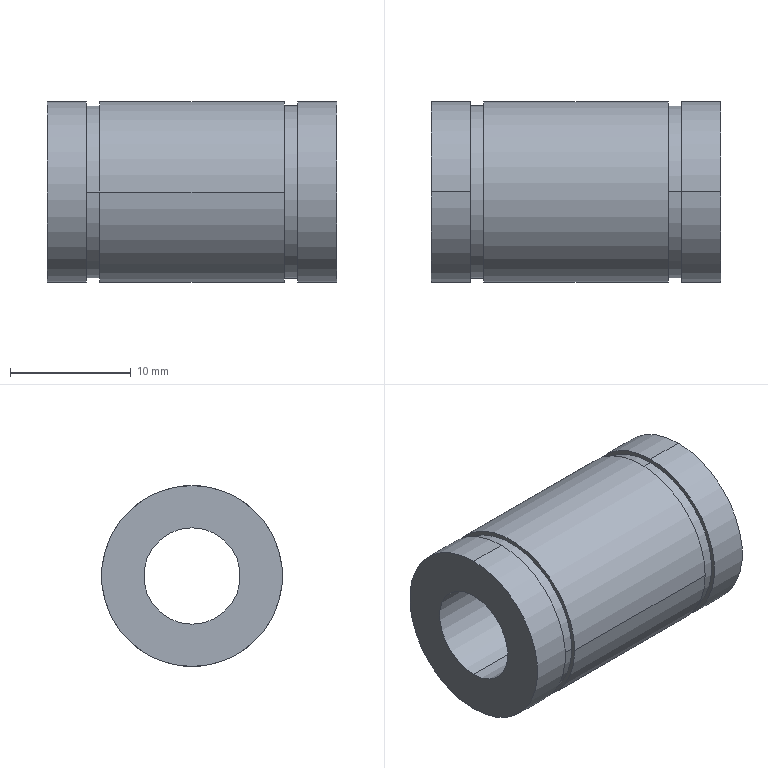Part | STEP file | Linear bearing LMU8 | 1 solid | 18 faces | box 24 x 15 x 15 mm | volume 2999 mm3 | cylinder 12 | plane 6 | commonest cylinder face diameters 15 x6 14.3 x4 8 x2
STEP:
#1=CARTESIAN_POINT('',(0.,0.,0.));
#2=DIRECTION('',(0.,0.,1.));
#3=DIRECTION('',(1.,0.,0.));
#4=AXIS2_PLACEMENT_3D('',#1,#2,#3);
#5=CARTESIAN_POINT('',(8.75,0.,-7.15));
#6=VERTEX_POINT('',#5);
#7=CARTESIAN_POINT('',(8.75,0.,7.15));
#8=VERTEX_POINT('',#7);
#9=CARTESIAN_POINT('',(8.75,0.,0.));
#10=DIRECTION('',(1.,0.,0.));
#11=DIRECTION('',(0.,0.,1.));
#12=AXIS2_PLACEMENT_3D('',#9,#10,#11);
#13=CIRCLE('',#12,7.15);
#14=CARTESIAN_POINT('',(8.75,0.,0.));
#15=DIRECTION('',(-1.,0.,0.));
#16=DIRECTION('',(0.,0.,1.));
#17=AXIS2_PLACEMENT_3D('',#14,#15,#16);
#18=CYLINDRICAL_SURFACE('',#17,7.15);
#19=CARTESIAN_POINT('',(6.283,0.));
#20=DIRECTION('',(-1.,0.));
#21=VECTOR('',#20,1.);
#22=LINE('',#19,#21);
#23=(GEOMETRIC_REPRESENTATION_CONTEXT(2)PARAMETRIC_REPRESENTATION_CONTEXT()REPRESENTATION_CONTEXT('',''));
#24=DEFINITIONAL_REPRESENTATION('',(#22),#23);
#25=PCURVE('',#18,#24);
#26=CARTESIAN_POINT('',(8.75,-7.59,-7.59));
#27=DIRECTION('',(-1.,0.,0.));
#28=DIRECTION('',(0.,0.,1.));
#29=AXIS2_PLACEMENT_3D('',#26,#27,#28);
#30=PLANE('',#29);
#31=CARTESIAN_POINT('',(14.74,7.59));
#32=CARTESIAN_POINT('',(14.74,-4.794));
#33=CARTESIAN_POINT('',(4.015,1.398));
#34=CARTESIAN_POINT('',(-6.71,7.59));
#35=CARTESIAN_POINT('',(4.015,13.782));
#36=CARTESIAN_POINT('',(14.74,19.974));
#37=CARTESIAN_POINT('',(14.74,7.59));
#38=(BOUNDED_CURVE()B_SPLINE_CURVE(2,(#31,#32,#33,#34,#35,#36,#37),.UNSPECIFIED.,.T.,.F.)B_SPLINE_CURVE_WITH_KNOTS((1,2,2,2,2,1),(-2.094,0.,2.094,4.189,6.283,8.378),.UNSPECIFIED.)CURVE()GEOMETRIC_REPRESENTATION_ITEM()RATIONAL_B_SPLINE_CURVE((1.,0.5,1.,0.5,1.,0.5,1.))REPRESENTATION_ITEM(''));
#39=(GEOMETRIC_REPRESENTATION_CONTEXT(2)PARAMETRIC_REPRESENTATION_CONTEXT()REPRESENTATION_CONTEXT('',''));
#40=DEFINITIONAL_REPRESENTATION('',(#38),#39);
#41=PCURVE('',#30,#40);
#42=SURFACE_CURVE('',#13,(#25,#41),.PCURVE_S1.);
#43=EDGE_CURVE('',#6,#8,#42,.T.);
#44=ORIENTED_EDGE('',*,*,#43,.F.);
#45=CARTESIAN_POINT('',(7.65,0.,-7.15));
#46=VERTEX_POINT('',#45);
#47=CARTESIAN_POINT('',(8.75,0.,-7.15));
#48=DIRECTION('',(-1.,0.,0.));
#49=VECTOR('',#48,1.);
#50=LINE('',#47,#49);
#51=CARTESIAN_POINT('',(3.142,0.));
#52=DIRECTION('',(0.,1.));
#53=VECTOR('',#52,1.);
#54=LINE('',#51,#53);
#55=(GEOMETRIC_REPRESENTATION_CONTEXT(2)PARAMETRIC_REPRESENTATION_CONTEXT()REPRESENTATION_CONTEXT('',''));
#56=DEFINITIONAL_REPRESENTATION('',(#54),#55);
#57=PCURVE('',#18,#56);
#58=CARTESIAN_POINT('',(8.75,0.,0.));
#59=DIRECTION('',(-1.,0.,0.));
#60=DIRECTION('',(0.,0.,1.));
#61=AXIS2_PLACEMENT_3D('',#58,#59,#60);
#62=CYLINDRICAL_SURFACE('',#61,7.15);
#63=CARTESIAN_POINT('',(3.142,0.));
#64=DIRECTION('',(0.,1.));
#65=VECTOR('',#64,1.);
#66=LINE('',#63,#65);
#67=(GEOMETRIC_REPRESENTATION_CONTEXT(2)PARAMETRIC_REPRESENTATION_CONTEXT()REPRESENTATION_CONTEXT('',''));
#68=DEFINITIONAL_REPRESENTATION('',(#66),#67);
#69=PCURVE('',#62,#68);
#70=SURFACE_CURVE('',#50,(#57,#69),.PCURVE_S1.);
#71=EDGE_CURVE('',#6,#46,#70,.T.);
#72=ORIENTED_EDGE('',*,*,#71,.T.);
#73=CARTESIAN_POINT('',(7.65,0.,7.15));
#74=VERTEX_POINT('',#73);
#75=CARTESIAN_POINT('',(7.65,0.,0.));
#76=DIRECTION('',(-1.,0.,0.));
#77=DIRECTION('',(0.,0.,1.));
#78=AXIS2_PLACEMENT_3D('',#75,#76,#77);
#79=CIRCLE('',#78,7.15);
#80=CARTESIAN_POINT('',(0.,1.1));
#81=DIRECTION('',(1.,0.));
#82=VECTOR('',#81,1.);
#83=LINE('',#80,#82);
#84=(GEOMETRIC_REPRESENTATION_CONTEXT(2)PARAMETRIC_REPRESENTATION_CONTEXT()REPRESENTATION_CONTEXT('',''));
#85=DEFINITIONAL_REPRESENTATION('',(#83),#84);
#86=PCURVE('',#18,#85);
#87=CARTESIAN_POINT('',(7.65,-7.59,7.59));
#88=DIRECTION('',(1.,0.,0.));
#89=DIRECTION('',(0.,0.,-1.));
#90=AXIS2_PLACEMENT_3D('',#87,#88,#89);
#91=PLANE('',#90);
#92=CARTESIAN_POINT('',(0.44,7.59));
#93=CARTESIAN_POINT('',(0.44,19.974));
#94=CARTESIAN_POINT('',(11.165,13.782));
#95=CARTESIAN_POINT('',(21.89,7.59));
#96=CARTESIAN_POINT('',(11.165,1.398));
#97=CARTESIAN_POINT('',(0.44,-4.794));
#98=CARTESIAN_POINT('',(0.44,7.59));
#99=(BOUNDED_CURVE()B_SPLINE_CURVE(2,(#92,#93,#94,#95,#96,#97,#98),.UNSPECIFIED.,.T.,.F.)B_SPLINE_CURVE_WITH_KNOTS((1,2,2,2,2,1),(-2.094,0.,2.094,4.189,6.283,8.378),.UNSPECIFIED.)CURVE()GEOMETRIC_REPRESENTATION_ITEM()RATIONAL_B_SPLINE_CURVE((1.,0.5,1.,0.5,1.,0.5,1.))REPRESENTATION_ITEM(''));
#100=(GEOMETRIC_REPRESENTATION_CONTEXT(2)PARAMETRIC_REPRESENTATION_CONTEXT()REPRESENTATION_CONTEXT('',''));
#101=DEFINITIONAL_REPRESENTATION('',(#99),#100);
#102=PCURVE('',#91,#101);
#103=SURFACE_CURVE('',#79,(#86,#102),.PCURVE_S1.);
#104=EDGE_CURVE('',#74,#46,#103,.T.);
#105=ORIENTED_EDGE('',*,*,#104,.F.);
#106=CARTESIAN_POINT('',(8.75,0.,7.15));
#107=DIRECTION('',(-1.,0.,0.));
#108=VECTOR('',#107,1.);
#109=LINE('',#106,#108);
#110=CARTESIAN_POINT('',(0.,0.));
#111=DIRECTION('',(0.,1.));
#112=VECTOR('',#111,1.);
#113=LINE('',#110,#112);
#114=(GEOMETRIC_REPRESENTATION_CONTEXT(2)PARAMETRIC_REPRESENTATION_CONTEXT()REPRESENTATION_CONTEXT('',''));
#115=DEFINITIONAL_REPRESENTATION('',(#113),#114);
#116=PCURVE('',#18,#115);
#117=CARTESIAN_POINT('',(6.283,0.));
#118=DIRECTION('',(0.,1.));
#119=VECTOR('',#118,1.);
#120=LINE('',#117,#119);
#121=(GEOMETRIC_REPRESENTATION_CONTEXT(2)PARAMETRIC_REPRESENTATION_CONTEXT()REPRESENTATION_CONTEXT('',''));
#122=DEFINITIONAL_REPRESENTATION('',(#120),#121);
#123=PCURVE('',#62,#122);
#124=SURFACE_CURVE('',#109,(#116,#123),.PCURVE_S1.);
#125=EDGE_CURVE('',#8,#74,#124,.T.);
#126=ORIENTED_EDGE('',*,*,#125,.F.);
#127=EDGE_LOOP('',(#44,#72,#105,#126));
#128=FACE_BOUND('',#127,.T.);
#129=ADVANCED_FACE('',(#128),#18,.T.);
#130=CARTESIAN_POINT('',(12.,0.,-7.5));
#131=VERTEX_POINT('',#130);
#132=CARTESIAN_POINT('',(12.,0.,7.5));
#133=VERTEX_POINT('',#132);
#134=CARTESIAN_POINT('',(12.,0.,0.));
#135=DIRECTION('',(1.,0.,0.));
#136=DIRECTION('',(0.,0.,1.));
#137=AXIS2_PLACEMENT_3D('',#134,#135,#136);
#138=CIRCLE('',#137,7.5);
#139=CARTESIAN_POINT('',(12.,0.,0.));
#140=DIRECTION('',(-1.,0.,0.));
#141=DIRECTION('',(0.,0.,1.));
#142=AXIS2_PLACEMENT_3D('',#139,#140,#141);
#143=CYLINDRICAL_SURFACE('',#142,7.5);
#144=CARTESIAN_POINT('',(6.283,0.));
#145=DIRECTION('',(-1.,0.));
#146=VECTOR('',#145,1.);
#147=LINE('',#144,#146);
#148=(GEOMETRIC_REPRESENTATION_CONTEXT(2)PARAMETRIC_REPRESENTATION_CONTEXT()REPRESENTATION_CONTEXT('',''));
#149=DEFINITIONAL_REPRESENTATION('',(#147),#148);
#150=PCURVE('',#143,#149);
#151=CARTESIAN_POINT('',(12.,-7.59,7.59));
#152=DIRECTION('',(1.,0.,0.));
#153=DIRECTION('',(0.,0.,-1.));
#154=AXIS2_PLACEMENT_3D('',#151,#152,#153);
#155=PLANE('',#154);
#156=CARTESIAN_POINT('',(7.59,7.59));
#157=DIRECTION('',(-1.,0.));
#158=AXIS2_PLACEMENT_2D('',#156,#157);
#159=CIRCLE('',#158,7.5);
#160=(GEOMETRIC_REPRESENTATION_CONTEXT(2)PARAMETRIC_REPRESENTATION_CONTEXT()REPRESENTATION_CONTEXT('',''));
#161=DEFINITIONAL_REPRESENTATION('',(#159),#160);
#162=PCURVE('',#155,#161);
#163=SURFACE_CURVE('',#138,(#150,#162),.PCURVE_S1.);
#164=EDGE_CURVE('',#131,#133,#163,.T.);
#165=ORIENTED_EDGE('',*,*,#164,.F.);
#166=CARTESIAN_POINT('',(8.75,0.,-7.5));
#167=VERTEX_POINT('',#166);
#168=CARTESIAN_POINT('',(12.,0.,-7.5));
#169=DIRECTION('',(-1.,0.,0.));
#170=VECTOR('',#169,1.);
#171=LINE('',#168,#170);
#172=CARTESIAN_POINT('',(3.142,0.));
#173=DIRECTION('',(0.,1.));
#174=VECTOR('',#173,1.);
#175=LINE('',#172,#174);
#176=(GEOMETRIC_REPRESENTATION_CONTEXT(2)PARAMETRIC_REPRESENTATION_CONTEXT()REPRESENTATION_CONTEXT('',''));
#177=DEFINITIONAL_REPRESENTATION('',(#175),#176);
#178=PCURVE('',#143,#177);
#179=CARTESIAN_POINT('',(12.,0.,0.));
#180=DIRECTION('',(-1.,0.,0.));
#181=DIRECTION('',(0.,0.,1.));
#182=AXIS2_PLACEMENT_3D('',#179,#180,#181);
#183=CYLINDRICAL_SURFACE('',#182,7.5);
#184=CARTESIAN_POINT('',(3.142,0.));
#185=DIRECTION('',(0.,1.));
#186=VECTOR('',#185,1.);
#187=LINE('',#184,#186);
#188=(GEOMETRIC_REPRESENTATION_CONTEXT(2)PARAMETRIC_REPRESENTATION_CONTEXT()REPRESENTATION_CONTEXT('',''));
#189=DEFINITIONAL_REPRESENTATION('',(#187),#188);
#190=PCURVE('',#183,#189);
#191=SURFACE_CURVE('',#171,(#178,#190),.PCURVE_S1.);
#192=EDGE_CURVE('',#131,#167,#191,.T.);
#193=ORIENTED_EDGE('',*,*,#192,.T.);
#194=CARTESIAN_POINT('',(8.75,0.,7.5));
#195=VERTEX_POINT('',#194);
#196=CARTESIAN_POINT('',(8.75,0.,0.));
#197=DIRECTION('',(-1.,0.,0.));
#198=DIRECTION('',(0.,0.,1.));
#199=AXIS2_PLACEMENT_3D('',#196,#197,#198);
#200=CIRCLE('',#199,7.5);
#201=CARTESIAN_POINT('',(0.,3.25));
#202=DIRECTION('',(1.,0.));
#203=VECTOR('',#202,1.);
#204=LINE('',#201,#203);
#205=(GEOMETRIC_REPRESENTATION_CONTEXT(2)PARAMETRIC_REPRESENTATION_CONTEXT()REPRESENTATION_CONTEXT('',''));
#206=DEFINITIONAL_REPRESENTATION('',(#204),#205);
#207=PCURVE('',#143,#206);
#208=CARTESIAN_POINT('',(7.59,7.59));
#209=DIRECTION('',(1.,0.));
#210=AXIS2_PLACEMENT_2D('',#208,#209);
#211=CIRCLE('',#210,7.5);
#212=(GEOMETRIC_REPRESENTATION_CONTEXT(2)PARAMETRIC_REPRESENTATION_CONTEXT()REPRESENTATION_CONTEXT('',''));
#213=DEFINITIONAL_REPRESENTATION('',(#211),#212);
#214=PCURVE('',#30,#213);
#215=SURFACE_CURVE('',#200,(#207,#214),.PCURVE_S1.);
#216=EDGE_CURVE('',#195,#167,#215,.T.);
#217=ORIENTED_EDGE('',*,*,#216,.F.);
#218=CARTESIAN_POINT('',(12.,0.,7.5));
#219=DIRECTION('',(-1.,0.,0.));
#220=VECTOR('',#219,1.);
#221=LINE('',#218,#220);
#222=CARTESIAN_POINT('',(0.,0.));
#223=DIRECTION('',(0.,1.));
#224=VECTOR('',#223,1.);
#225=LINE('',#222,#224);
#226=(GEOMETRIC_REPRESENTATION_CONTEXT(2)PARAMETRIC_REPRESENTATION_CONTEXT()REPRESENTATION_CONTEXT('',''));
#227=DEFINITIONAL_REPRESENTATION('',(#225),#226);
#228=PCURVE('',#143,#227);
#229=CARTESIAN_POINT('',(6.283,0.));
#230=DIRECTION('',(0.,1.));
#231=VECTOR('',#230,1.);
#232=LINE('',#229,#231);
#233=(GEOMETRIC_REPRESENTATION_CONTEXT(2)PARAMETRIC_REPRESENTATION_CONTEXT()REPRESENTATION_CONTEXT('',''));
#234=DEFINITIONAL_REPRESENTATION('',(#232),#233);
#235=PCURVE('',#183,#234);
#236=SURFACE_CURVE('',#221,(#228,#235),.PCURVE_S1.);
#237=EDGE_CURVE('',#133,#195,#236,.T.);
#238=ORIENTED_EDGE('',*,*,#237,.F.);
#239=EDGE_LOOP('',(#165,#193,#217,#238));
#240=FACE_BOUND('',#239,.T.);
#241=ADVANCED_FACE('',(#240),#143,.T.);
#242=CARTESIAN_POINT('',(7.65,7.5,0.));
#243=VERTEX_POINT('',#242);
#244=CARTESIAN_POINT('',(7.65,-7.5,0.));
#245=VERTEX_POINT('',#244);
#246=CARTESIAN_POINT('',(7.65,0.,0.));
#247=DIRECTION('',(1.,0.,0.));
#248=DIRECTION('',(0.,-1.,0.));
#249=AXIS2_PLACEMENT_3D('',#246,#247,#248);
#250=CIRCLE('',#249,7.5);
#251=CARTESIAN_POINT('',(7.65,0.,0.));
#252=DIRECTION('',(-1.,0.,0.));
#253=DIRECTION('',(0.,-1.,0.));
#254=AXIS2_PLACEMENT_3D('',#251,#252,#253);
#255=CYLINDRICAL_SURFACE('',#254,7.5);
#256=CARTESIAN_POINT('',(6.283,0.));
#257=DIRECTION('',(-1.,0.));
#258=VECTOR('',#257,1.);
#259=LINE('',#256,#258);
#260=(GEOMETRIC_REPRESENTATION_CONTEXT(2)PARAMETRIC_REPRESENTATION_CONTEXT()REPRESENTATION_CONTEXT('',''));
#261=DEFINITIONAL_REPRESENTATION('',(#259),#260);
#262=PCURVE('',#255,#261);
#263=CARTESIAN_POINT('',(7.59,7.59));
#264=DIRECTION('',(0.,-1.));
#265=AXIS2_PLACEMENT_2D('',#263,#264);
#266=CIRCLE('',#265,7.5);
#267=(GEOMETRIC_REPRESENTATION_CONTEXT(2)PARAMETRIC_REPRESENTATION_CONTEXT()REPRESENTATION_CONTEXT('',''));
#268=DEFINITIONAL_REPRESENTATION('',(#266),#267);
#269=PCURVE('',#91,#268);
#270=SURFACE_CURVE('',#250,(#262,#269),.PCURVE_S1.);
#271=EDGE_CURVE('',#243,#245,#270,.T.);
#272=ORIENTED_EDGE('',*,*,#271,.F.);
#273=CARTESIAN_POINT('',(-7.65,7.5,0.));
#274=VERTEX_POINT('',#273);
#275=CARTESIAN_POINT('',(7.65,7.5,0.));
#276=DIRECTION('',(-1.,0.,0.));
#277=VECTOR('',#276,1.);
#278=LINE('',#275,#277);
#279=CARTESIAN_POINT('',(3.142,0.));
#280=DIRECTION('',(0.,1.));
#281=VECTOR('',#280,1.);
#282=LINE('',#279,#281);
#283=(GEOMETRIC_REPRESENTATION_CONTEXT(2)PARAMETRIC_REPRESENTATION_CONTEXT()REPRESENTATION_CONTEXT('',''));
#284=DEFINITIONAL_REPRESENTATION('',(#282),#283);
#285=PCURVE('',#255,#284);
#286=CARTESIAN_POINT('',(7.65,0.,0.));
#287=DIRECTION('',(-1.,0.,0.));
#288=DIRECTION('',(0.,-1.,0.));
#289=AXIS2_PLACEMENT_3D('',#286,#287,#288);
#290=CYLINDRICAL_SURFACE('',#289,7.5);
#291=CARTESIAN_POINT('',(3.142,0.));
#292=DIRECTION('',(0.,1.));
#293=VECTOR('',#292,1.);
#294=LINE('',#291,#293);
#295=(GEOMETRIC_REPRESENTATION_CONTEXT(2)PARAMETRIC_REPRESENTATION_CONTEXT()REPRESENTATION_CONTEXT('',''));
#296=DEFINITIONAL_REPRESENTATION('',(#294),#295);
#297=PCURVE('',#290,#296);
#298=SURFACE_CURVE('',#278,(#285,#297),.PCURVE_S1.);
#299=EDGE_CURVE('',#243,#274,#298,.T.);
#300=ORIENTED_EDGE('',*,*,#299,.T.);
#301=CARTESIAN_POINT('',(-7.65,-7.5,0.));
#302=VERTEX_POINT('',#301);
#303=CARTESIAN_POINT('',(-7.65,0.,0.));
#304=DIRECTION('',(-1.,0.,0.));
#305=DIRECTION('',(0.,-1.,0.));
#306=AXIS2_PLACEMENT_3D('',#303,#304,#305);
#307=CIRCLE('',#306,7.5);
#308=CARTESIAN_POINT('',(0.,15.3));
#309=DIRECTION('',(1.,0.));
#310=VECTOR('',#309,1.);
#311=LINE('',#308,#310);
#312=(GEOMETRIC_REPRESENTATION_CONTEXT(2)PARAMETRIC_REPRESENTATION_CONTEXT()REPRESENTATION_CONTEXT('',''));
#313=DEFINITIONAL_REPRESENTATION('',(#311),#312);
#314=PCURVE('',#255,#313);
#315=CARTESIAN_POINT('',(-7.65,-7.59,-7.59));
#316=DIRECTION('',(-1.,0.,0.));
#317=DIRECTION('',(0.,0.,1.));
#318=AXIS2_PLACEMENT_3D('',#315,#316,#317);
#319=PLANE('',#318);
#320=CARTESIAN_POINT('',(7.59,7.59));
#321=DIRECTION('',(0.,-1.));
#322=AXIS2_PLACEMENT_2D('',#320,#321);
#323=CIRCLE('',#322,7.5);
#324=(GEOMETRIC_REPRESENTATION_CONTEXT(2)PARAMETRIC_REPRESENTATION_CONTEXT()REPRESENTATION_CONTEXT('',''));
#325=DEFINITIONAL_REPRESENTATION('',(#323),#324);
#326=PCURVE('',#319,#325);
#327=SURFACE_CURVE('',#307,(#314,#326),.PCURVE_S1.);
#328=EDGE_CURVE('',#302,#274,#327,.T.);
#329=ORIENTED_EDGE('',*,*,#328,.F.);
#330=CARTESIAN_POINT('',(7.65,-7.5,0.));
#331=DIRECTION('',(-1.,0.,0.));
#332=VECTOR('',#331,1.);
#333=LINE('',#330,#332);
#334=CARTESIAN_POINT('',(0.,0.));
#335=DIRECTION('',(0.,1.));
#336=VECTOR('',#335,1.);
#337=LINE('',#334,#336);
#338=(GEOMETRIC_REPRESENTATION_CONTEXT(2)PARAMETRIC_REPRESENTATION_CONTEXT()REPRESENTATION_CONTEXT('',''));
#339=DEFINITIONAL_REPRESENTATION('',(#337),#338);
#340=PCURVE('',#255,#339);
#341=CARTESIAN_POINT('',(6.283,0.));
#342=DIRECTION('',(0.,1.));
#343=VECTOR('',#342,1.);
#344=LINE('',#341,#343);
#345=(GEOMETRIC_REPRESENTATION_CONTEXT(2)PARAMETRIC_REPRESENTATION_CONTEXT()REPRESENTATION_CONTEXT('',''));
#346=DEFINITIONAL_REPRESENTATION('',(#344),#345);
#347=PCURVE('',#290,#346);
#348=SURFACE_CURVE('',#333,(#340,#347),.PCURVE_S1.);
#349=EDGE_CURVE('',#245,#302,#348,.T.);
#350=ORIENTED_EDGE('',*,*,#349,.F.);
#351=EDGE_LOOP('',(#272,#300,#329,#350));
#352=FACE_BOUND('',#351,.T.);
#353=ADVANCED_FACE('',(#352),#255,.T.);
#354=CARTESIAN_POINT('',(12.,0.,4.));
#355=VERTEX_POINT('',#354);
#356=CARTESIAN_POINT('',(-12.,0.,4.));
#357=VERTEX_POINT('',#356);
#358=CARTESIAN_POINT('',(12.,0.,4.));
#359=DIRECTION('',(-1.,0.,0.));
#360=VECTOR('',#359,1.);
#361=LINE('',#358,#360);
#362=CARTESIAN_POINT('',(12.,0.,0.));
#363=DIRECTION('',(-1.,0.,0.));
#364=DIRECTION('',(0.,0.,1.));
#365=AXIS2_PLACEMENT_3D('',#362,#363,#364);
#366=CYLINDRICAL_SURFACE('',#365,4.);
#367=CARTESIAN_POINT('',(6.283,0.));
#368=DIRECTION('',(0.,1.));
#369=VECTOR('',#368,1.);
#370=LINE('',#367,#369);
#371=(GEOMETRIC_REPRESENTATION_CONTEXT(2)PARAMETRIC_REPRESENTATION_CONTEXT()REPRESENTATION_CONTEXT('',''));
#372=DEFINITIONAL_REPRESENTATION('',(#370),#371);
#373=PCURVE('',#366,#372);
#374=CARTESIAN_POINT('',(12.,0.,0.));
#375=DIRECTION('',(-1.,0.,0.));
#376=DIRECTION('',(0.,0.,1.));
#377=AXIS2_PLACEMENT_3D('',#374,#375,#376);
#378=CYLINDRICAL_SURFACE('',#377,4.);
#379=CARTESIAN_POINT('',(0.,0.));
#380=DIRECTION('',(0.,1.));
#381=VECTOR('',#380,1.);
#382=LINE('',#379,#381);
#383=(GEOMETRIC_REPRESENTATION_CONTEXT(2)PARAMETRIC_REPRESENTATION_CONTEXT()REPRESENTATION_CONTEXT('',''));
#384=DEFINITIONAL_REPRESENTATION('',(#382),#383);
#385=PCURVE('',#378,#384);
#386=SURFACE_CURVE('',#361,(#373,#385),.PCURVE_S1.);
#387=EDGE_CURVE('',#355,#357,#386,.T.);
#388=ORIENTED_EDGE('',*,*,#387,.T.);
#389=CARTESIAN_POINT('',(-12.,0.,-4.));
#390=VERTEX_POINT('',#389);
#391=CARTESIAN_POINT('',(-12.,0.,0.));
#392=DIRECTION('',(-1.,0.,0.));
#393=DIRECTION('',(0.,0.,1.));
#394=AXIS2_PLACEMENT_3D('',#391,#392,#393);
#395=CIRCLE('',#394,4.);
#396=CARTESIAN_POINT('',(0.,24.));
#397=DIRECTION('',(1.,0.));
#398=VECTOR('',#397,1.);
#399=LINE('',#396,#398);
#400=(GEOMETRIC_REPRESENTATION_CONTEXT(2)PARAMETRIC_REPRESENTATION_CONTEXT()REPRESENTATION_CONTEXT('',''));
#401=DEFINITIONAL_REPRESENTATION('',(#399),#400);
#402=PCURVE('',#366,#401);
#403=CARTESIAN_POINT('',(-12.,-7.59,7.59));
#404=DIRECTION('',(1.,0.,0.));
#405=DIRECTION('',(0.,0.,-1.));
#406=AXIS2_PLACEMENT_3D('',#403,#404,#405);
#407=PLANE('',#406);
#408=CARTESIAN_POINT('',(3.59,7.59));
#409=CARTESIAN_POINT('',(3.59,14.518));
#410=CARTESIAN_POINT('',(9.59,11.054));
#411=CARTESIAN_POINT('',(15.59,7.59));
#412=CARTESIAN_POINT('',(9.59,4.126));
#413=CARTESIAN_POINT('',(3.59,0.6618));
#414=CARTESIAN_POINT('',(3.59,7.59));
#415=(BOUNDED_CURVE()B_SPLINE_CURVE(2,(#408,#409,#410,#411,#412,#413,#414),.UNSPECIFIED.,.T.,.F.)B_SPLINE_CURVE_WITH_KNOTS((1,2,2,2,2,1),(-2.094,0.,2.094,4.189,6.283,8.378),.UNSPECIFIED.)CURVE()GEOMETRIC_REPRESENTATION_ITEM()RATIONAL_B_SPLINE_CURVE((1.,0.5,1.,0.5,1.,0.5,1.))REPRESENTATION_ITEM(''));
#416=(GEOMETRIC_REPRESENTATION_CONTEXT(2)PARAMETRIC_REPRESENTATION_CONTEXT()REPRESENTATION_CONTEXT('',''));
#417=DEFINITIONAL_REPRESENTATION('',(#415),#416);
#418=PCURVE('',#407,#417);
#419=SURFACE_CURVE('',#395,(#402,#418),.PCURVE_S1.);
#420=EDGE_CURVE('',#390,#357,#419,.T.);
#421=ORIENTED_EDGE('',*,*,#420,.F.);
#422=CARTESIAN_POINT('',(12.,0.,-4.));
#423=VERTEX_POINT('',#422);
#424=CARTESIAN_POINT('',(12.,0.,-4.));
#425=DIRECTION('',(-1.,0.,0.));
#426=VECTOR('',#425,1.);
#427=LINE('',#424,#426);
#428=CARTESIAN_POINT('',(3.142,0.));
#429=DIRECTION('',(0.,1.));
#430=VECTOR('',#429,1.);
#431=LINE('',#428,#430);
#432=(GEOMETRIC_REPRESENTATION_CONTEXT(2)PARAMETRIC_REPRESENTATION_CONTEXT()REPRESENTATION_CONTEXT('',''));
#433=DEFINITIONAL_REPRESENTATION('',(#431),#432);
#434=PCURVE('',#366,#433);
#435=CARTESIAN_POINT('',(3.142,0.));
#436=DIRECTION('',(0.,1.));
#437=VECTOR('',#436,1.);
#438=LINE('',#435,#437);
#439=(GEOMETRIC_REPRESENTATION_CONTEXT(2)PARAMETRIC_REPRESENTATION_CONTEXT()REPRESENTATION_CONTEXT('',''));
#440=DEFINITIONAL_REPRESENTATION('',(#438),#439);
#441=PCURVE('',#378,#440);
#442=SURFACE_CURVE('',#427,(#434,#441),.PCURVE_S1.);
#443=EDGE_CURVE('',#423,#390,#442,.T.);
#444=ORIENTED_EDGE('',*,*,#443,.F.);
#445=CARTESIAN_POINT('',(12.,0.,0.));
#446=DIRECTION('',(-1.,0.,0.));
#447=DIRECTION('',(0.,0.,1.));
#448=AXIS2_PLACEMENT_3D('',#445,#446,#447);
#449=CIRCLE('',#448,4.);
#450=CARTESIAN_POINT('',(0.,0.));
#451=DIRECTION('',(1.,0.));
#452=VECTOR('',#451,1.);
#453=LINE('',#450,#452);
#454=(GEOMETRIC_REPRESENTATION_CONTEXT(2)PARAMETRIC_REPRESENTATION_CONTEXT()REPRESENTATION_CONTEXT('',''));
#455=DEFINITIONAL_REPRESENTATION('',(#453),#454);
#456=PCURVE('',#366,#455);
#457=CARTESIAN_POINT('',(3.59,7.59));
#458=CARTESIAN_POINT('',(3.59,14.518));
#459=CARTESIAN_POINT('',(9.59,11.054));
#460=CARTESIAN_POINT('',(15.59,7.59));
#461=CARTESIAN_POINT('',(9.59,4.126));
#462=CARTESIAN_POINT('',(3.59,0.6618));
#463=CARTESIAN_POINT('',(3.59,7.59));
#464=(BOUNDED_CURVE()B_SPLINE_CURVE(2,(#457,#458,#459,#460,#461,#462,#463),.UNSPECIFIED.,.T.,.F.)B_SPLINE_CURVE_WITH_KNOTS((1,2,2,2,2,1),(-2.094,0.,2.094,4.189,6.283,8.378),.UNSPECIFIED.)CURVE()GEOMETRIC_REPRESENTATION_ITEM()RATIONAL_B_SPLINE_CURVE((1.,0.5,1.,0.5,1.,0.5,1.))REPRESENTATION_ITEM(''));
#465=(GEOMETRIC_REPRESENTATION_CONTEXT(2)PARAMETRIC_REPRESENTATION_CONTEXT()REPRESENTATION_CONTEXT('',''));
#466=DEFINITIONAL_REPRESENTATION('',(#464),#465);
#467=PCURVE('',#155,#466);
#468=SURFACE_CURVE('',#449,(#456,#467),.PCURVE_S1.);
#469=EDGE_CURVE('',#423,#355,#468,.T.);
#470=ORIENTED_EDGE('',*,*,#469,.T.);
#471=EDGE_LOOP('',(#388,#421,#444,#470));
#472=FACE_BOUND('',#471,.F.);
#473=ADVANCED_FACE('',(#472),#366,.F.);
#474=CARTESIAN_POINT('',(-7.65,7.15,0.));
#475=VERTEX_POINT('',#474);
#476=CARTESIAN_POINT('',(-7.65,-7.15,0.));
#477=VERTEX_POINT('',#476);
#478=CARTESIAN_POINT('',(-7.65,0.,0.));
#479=DIRECTION('',(1.,0.,0.));
#480=DIRECTION('',(0.,-1.,0.));
#481=AXIS2_PLACEMENT_3D('',#478,#479,#480);
#482=CIRCLE('',#481,7.15);
#483=CARTESIAN_POINT('',(-7.65,0.,0.));
#484=DIRECTION('',(-1.,0.,0.));
#485=DIRECTION('',(0.,-1.,0.));
#486=AXIS2_PLACEMENT_3D('',#483,#484,#485);
#487=CYLINDRICAL_SURFACE('',#486,7.15);
#488=CARTESIAN_POINT('',(6.283,0.));
#489=DIRECTION('',(-1.,0.));
#490=VECTOR('',#489,1.);
#491=LINE('',#488,#490);
#492=(GEOMETRIC_REPRESENTATION_CONTEXT(2)PARAMETRIC_REPRESENTATION_CONTEXT()REPRESENTATION_CONTEXT('',''));
#493=DEFINITIONAL_REPRESENTATION('',(#491),#492);
#494=PCURVE('',#487,#493);
#495=CARTESIAN_POINT('',(7.59,0.44));
#496=CARTESIAN_POINT('',(-4.794,0.44));
#497=CARTESIAN_POINT('',(1.398,11.165));
#498=CARTESIAN_POINT('',(7.59,21.89));
#499=CARTESIAN_POINT('',(13.782,11.165));
#500=CARTESIAN_POINT('',(19.974,0.44));
#501=CARTESIAN_POINT('',(7.59,0.44));
#502=(BOUNDED_CURVE()B_SPLINE_CURVE(2,(#495,#496,#497,#498,#499,#500,#501),.UNSPECIFIED.,.T.,.F.)B_SPLINE_CURVE_WITH_KNOTS((1,2,2,2,2,1),(-2.094,0.,2.094,4.189,6.283,8.378),.UNSPECIFIED.)CURVE()GEOMETRIC_REPRESENTATION_ITEM()RATIONAL_B_SPLINE_CURVE((1.,0.5,1.,0.5,1.,0.5,1.))REPRESENTATION_ITEM(''));
#503=(GEOMETRIC_REPRESENTATION_CONTEXT(2)PARAMETRIC_REPRESENTATION_CONTEXT()REPRESENTATION_CONTEXT('',''));
#504=DEFINITIONAL_REPRESENTATION('',(#502),#503);
#505=PCURVE('',#319,#504);
#506=SURFACE_CURVE('',#482,(#494,#505),.PCURVE_S1.);
#507=EDGE_CURVE('',#475,#477,#506,.T.);
#508=ORIENTED_EDGE('',*,*,#507,.F.);
#509=CARTESIAN_POINT('',(-8.75,7.15,0.));
#510=VERTEX_POINT('',#509);
#511=CARTESIAN_POINT('',(-7.65,7.15,0.));
#512=DIRECTION('',(-1.,0.,0.));
#513=VECTOR('',#512,1.);
#514=LINE('',#511,#513);
#515=CARTESIAN_POINT('',(3.142,0.));
#516=DIRECTION('',(0.,1.));
#517=VECTOR('',#516,1.);
#518=LINE('',#515,#517);
#519=(GEOMETRIC_REPRESENTATION_CONTEXT(2)PARAMETRIC_REPRESENTATION_CONTEXT()REPRESENTATION_CONTEXT('',''));
#520=DEFINITIONAL_REPRESENTATION('',(#518),#519);
#521=PCURVE('',#487,#520);
#522=CARTESIAN_POINT('',(-7.65,0.,0.));
#523=DIRECTION('',(-1.,0.,0.));
#524=DIRECTION('',(0.,-1.,0.));
#525=AXIS2_PLACEMENT_3D('',#522,#523,#524);
#526=CYLINDRICAL_SURFACE('',#525,7.15);
#527=CARTESIAN_POINT('',(3.142,0.));
#528=DIRECTION('',(0.,1.));
#529=VECTOR('',#528,1.);
#530=LINE('',#527,#529);
#531=(GEOMETRIC_REPRESENTATION_CONTEXT(2)PARAMETRIC_REPRESENTATION_CONTEXT()REPRESENTATION_CONTEXT('',''));
#532=DEFINITIONAL_REPRESENTATION('',(#530),#531);
#533=PCURVE('',#526,#532);
#534=SURFACE_CURVE('',#514,(#521,#533),.PCURVE_S1.);
#535=EDGE_CURVE('',#475,#510,#534,.T.);
#536=ORIENTED_EDGE('',*,*,#535,.T.);
#537=CARTESIAN_POINT('',(-8.75,-7.15,0.));
#538=VERTEX_POINT('',#537);
#539=CARTESIAN_POINT('',(-8.75,0.,0.));
#540=DIRECTION('',(-1.,0.,0.));
#541=DIRECTION('',(0.,-1.,0.));
#542=AXIS2_PLACEMENT_3D('',#539,#540,#541);
#543=CIRCLE('',#542,7.15);
#544=CARTESIAN_POINT('',(0.,1.1));
#545=DIRECTION('',(1.,0.));
#546=VECTOR('',#545,1.);
#547=LINE('',#544,#546);
#548=(GEOMETRIC_REPRESENTATION_CONTEXT(2)PARAMETRIC_REPRESENTATION_CONTEXT()REPRESENTATION_CONTEXT('',''));
#549=DEFINITIONAL_REPRESENTATION('',(#547),#548);
#550=PCURVE('',#487,#549);
#551=CARTESIAN_POINT('',(-8.75,-7.59,7.59));
#552=DIRECTION('',(1.,0.,0.));
#553=DIRECTION('',(0.,0.,-1.));
#554=AXIS2_PLACEMENT_3D('',#551,#552,#553);
#555=PLANE('',#554);
#556=CARTESIAN_POINT('',(7.59,0.44));
#557=CARTESIAN_POINT('',(-4.794,0.44));
#558=CARTESIAN_POINT('',(1.398,11.165));
#559=CARTESIAN_POINT('',(7.59,21.89));
#560=CARTESIAN_POINT('',(13.782,11.165));
#561=CARTESIAN_POINT('',(19.974,0.44));
#562=CARTESIAN_POINT('',(7.59,0.44));
#563=(BOUNDED_CURVE()B_SPLINE_CURVE(2,(#556,#557,#558,#559,#560,#561,#562),.UNSPECIFIED.,.T.,.F.)B_SPLINE_CURVE_WITH_KNOTS((1,2,2,2,2,1),(-2.094,0.,2.094,4.189,6.283,8.378),.UNSPECIFIED.)CURVE()GEOMETRIC_REPRESENTATION_ITEM()RATIONAL_B_SPLINE_CURVE((1.,0.5,1.,0.5,1.,0.5,1.))REPRESENTATION_ITEM(''));
#564=(GEOMETRIC_REPRESENTATION_CONTEXT(2)PARAMETRIC_REPRESENTATION_CONTEXT()REPRESENTATION_CONTEXT('',''));
#565=DEFINITIONAL_REPRESENTATION('',(#563),#564);
#566=PCURVE('',#555,#565);
#567=SURFACE_CURVE('',#543,(#550,#566),.PCURVE_S1.);
#568=EDGE_CURVE('',#538,#510,#567,.T.);
#569=ORIENTED_EDGE('',*,*,#568,.F.);
#570=CARTESIAN_POINT('',(-7.65,-7.15,0.));
#571=DIRECTION('',(-1.,0.,0.));
#572=VECTOR('',#571,1.);
#573=LINE('',#570,#572);
#574=CARTESIAN_POINT('',(0.,0.));
#575=DIRECTION('',(0.,1.));
#576=VECTOR('',#575,1.);
#577=LINE('',#574,#576);
#578=(GEOMETRIC_REPRESENTATION_CONTEXT(2)PARAMETRIC_REPRESENTATION_CONTEXT()REPRESENTATION_CONTEXT('',''));
#579=DEFINITIONAL_REPRESENTATION('',(#577),#578);
#580=PCURVE('',#487,#579);
#581=CARTESIAN_POINT('',(6.283,0.));
#582=DIRECTION('',(0.,1.));
#583=VECTOR('',#582,1.);
#584=LINE('',#581,#583);
#585=(GEOMETRIC_REPRESENTATION_CONTEXT(2)PARAMETRIC_REPRESENTATION_CONTEXT()REPRESENTATION_CONTEXT('',''));
#586=DEFINITIONAL_REPRESENTATION('',(#584),#585);
#587=PCURVE('',#526,#586);
#588=SURFACE_CURVE('',#573,(#580,#587),.PCURVE_S1.);
#589=EDGE_CURVE('',#477,#538,#588,.T.);
#590=ORIENTED_EDGE('',*,*,#589,.F.);
#591=EDGE_LOOP('',(#508,#536,#569,#590));
#592=FACE_BOUND('',#591,.T.);
#593=ADVANCED_FACE('',(#592),#487,.T.);
#594=CARTESIAN_POINT('',(-8.75,0.,-7.5));
#595=VERTEX_POINT('',#594);
#596=CARTESIAN_POINT('',(-8.75,0.,7.5));
#597=VERTEX_POINT('',#596);
#598=CARTESIAN_POINT('',(-8.75,0.,0.));
#599=DIRECTION('',(1.,0.,0.));
#600=DIRECTION('',(0.,0.,1.));
#601=AXIS2_PLACEMENT_3D('',#598,#599,#600);
#602=CIRCLE('',#601,7.5);
#603=CARTESIAN_POINT('',(-8.75,0.,0.));
#604=DIRECTION('',(-1.,0.,0.));
#605=DIRECTION('',(0.,0.,1.));
#606=AXIS2_PLACEMENT_3D('',#603,#604,#605);
#607=CYLINDRICAL_SURFACE('',#606,7.5);
#608=CARTESIAN_POINT('',(6.283,0.));
#609=DIRECTION('',(-1.,0.));
#610=VECTOR('',#609,1.);
#611=LINE('',#608,#610);
#612=(GEOMETRIC_REPRESENTATION_CONTEXT(2)PARAMETRIC_REPRESENTATION_CONTEXT()REPRESENTATION_CONTEXT('',''));
#613=DEFINITIONAL_REPRESENTATION('',(#611),#612);
#614=PCURVE('',#607,#613);
#615=CARTESIAN_POINT('',(7.59,7.59));
#616=DIRECTION('',(-1.,0.));
#617=AXIS2_PLACEMENT_2D('',#615,#616);
#618=CIRCLE('',#617,7.5);
#619=(GEOMETRIC_REPRESENTATION_CONTEXT(2)PARAMETRIC_REPRESENTATION_CONTEXT()REPRESENTATION_CONTEXT('',''));
#620=DEFINITIONAL_REPRESENTATION('',(#618),#619);
#621=PCURVE('',#555,#620);
#622=SURFACE_CURVE('',#602,(#614,#621),.PCURVE_S1.);
#623=EDGE_CURVE('',#595,#597,#622,.T.);
#624=ORIENTED_EDGE('',*,*,#623,.F.);
#625=CARTESIAN_POINT('',(-12.,0.,-7.5));
#626=VERTEX_POINT('',#625);
#627=CARTESIAN_POINT('',(-8.75,0.,-7.5));
#628=DIRECTION('',(-1.,0.,0.));
#629=VECTOR('',#628,1.);
#630=LINE('',#627,#629);
#631=CARTESIAN_POINT('',(3.142,0.));
#632=DIRECTION('',(0.,1.));
#633=VECTOR('',#632,1.);
#634=LINE('',#631,#633);
#635=(GEOMETRIC_REPRESENTATION_CONTEXT(2)PARAMETRIC_REPRESENTATION_CONTEXT()REPRESENTATION_CONTEXT('',''));
#636=DEFINITIONAL_REPRESENTATION('',(#634),#635);
#637=PCURVE('',#607,#636);
#638=CARTESIAN_POINT('',(-8.75,0.,0.));
#639=DIRECTION('',(-1.,0.,0.));
#640=DIRECTION('',(0.,0.,1.));
#641=AXIS2_PLACEMENT_3D('',#638,#639,#640);
#642=CYLINDRICAL_SURFACE('',#641,7.5);
#643=CARTESIAN_POINT('',(3.142,0.));
#644=DIRECTION('',(0.,1.));
#645=VECTOR('',#644,1.);
#646=LINE('',#643,#645);
#647=(GEOMETRIC_REPRESENTATION_CONTEXT(2)PARAMETRIC_REPRESENTATION_CONTEXT()REPRESENTATION_CONTEXT('',''));
#648=DEFINITIONAL_REPRESENTATION('',(#646),#647);
#649=PCURVE('',#642,#648);
#650=SURFACE_CURVE('',#630,(#637,#649),.PCURVE_S1.);
#651=EDGE_CURVE('',#595,#626,#650,.T.);
#652=ORIENTED_EDGE('',*,*,#651,.T.);
#653=CARTESIAN_POINT('',(-12.,0.,7.5));
#654=VERTEX_POINT('',#653);
#655=CARTESIAN_POINT('',(-12.,0.,0.));
#656=DIRECTION('',(1.,0.,0.));
#657=DIRECTION('',(0.,0.,1.));
#658=AXIS2_PLACEMENT_3D('',#655,#656,#657);
#659=CIRCLE('',#658,7.5);
#660=CARTESIAN_POINT('',(6.283,3.25));
#661=DIRECTION('',(-1.,0.));
#662=VECTOR('',#661,1.);
#663=LINE('',#660,#662);
#664=(GEOMETRIC_REPRESENTATION_CONTEXT(2)PARAMETRIC_REPRESENTATION_CONTEXT()REPRESENTATION_CONTEXT('',''));
#665=DEFINITIONAL_REPRESENTATION('',(#663),#664);
#666=PCURVE('',#607,#665);
#667=CARTESIAN_POINT('',(7.59,7.59));
#668=DIRECTION('',(-1.,0.));
#669=AXIS2_PLACEMENT_2D('',#667,#668);
#670=CIRCLE('',#669,7.5);
#671=(GEOMETRIC_REPRESENTATION_CONTEXT(2)PARAMETRIC_REPRESENTATION_CONTEXT()REPRESENTATION_CONTEXT('',''));
#672=DEFINITIONAL_REPRESENTATION('',(#670),#671);
#673=PCURVE('',#407,#672);
#674=SURFACE_CURVE('',#659,(#666,#673),.PCURVE_S1.);
#675=EDGE_CURVE('',#626,#654,#674,.T.);
#676=ORIENTED_EDGE('',*,*,#675,.T.);
#677=CARTESIAN_POINT('',(-8.75,0.,7.5));
#678=DIRECTION('',(-1.,0.,0.));
#679=VECTOR('',#678,1.);
#680=LINE('',#677,#679);
#681=CARTESIAN_POINT('',(0.,0.));
#682=DIRECTION('',(0.,1.));
#683=VECTOR('',#682,1.);
#684=LINE('',#681,#683);
#685=(GEOMETRIC_REPRESENTATION_CONTEXT(2)PARAMETRIC_REPRESENTATION_CONTEXT()REPRESENTATION_CONTEXT('',''));
#686=DEFINITIONAL_REPRESENTATION('',(#684),#685);
#687=PCURVE('',#607,#686);
#688=CARTESIAN_POINT('',(6.283,0.));
#689=DIRECTION('',(0.,1.));
#690=VECTOR('',#689,1.);
#691=LINE('',#688,#690);
#692=(GEOMETRIC_REPRESENTATION_CONTEXT(2)PARAMETRIC_REPRESENTATION_CONTEXT()REPRESENTATION_CONTEXT('',''));
#693=DEFINITIONAL_REPRESENTATION('',(#691),#692);
#694=PCURVE('',#642,#693);
#695=SURFACE_CURVE('',#680,(#687,#694),.PCURVE_S1.);
#696=EDGE_CURVE('',#597,#654,#695,.T.);
#697=ORIENTED_EDGE('',*,*,#696,.F.);
#698=EDGE_LOOP('',(#624,#652,#676,#697));
#699=FACE_BOUND('',#698,.T.);
#700=ADVANCED_FACE('',(#699),#607,.T.);
#701=ORIENTED_EDGE('',*,*,#71,.F.);
#702=CARTESIAN_POINT('',(8.75,0.,0.));
#703=DIRECTION('',(1.,0.,0.));
#704=DIRECTION('',(0.,0.,1.));
#705=AXIS2_PLACEMENT_3D('',#702,#703,#704);
#706=CIRCLE('',#705,7.15);
#707=CARTESIAN_POINT('',(6.283,0.));
#708=DIRECTION('',(-1.,0.));
#709=VECTOR('',#708,1.);
#710=LINE('',#707,#709);
#711=(GEOMETRIC_REPRESENTATION_CONTEXT(2)PARAMETRIC_REPRESENTATION_CONTEXT()REPRESENTATION_CONTEXT('',''));
#712=DEFINITIONAL_REPRESENTATION('',(#710),#711);
#713=PCURVE('',#62,#712);
#714=CARTESIAN_POINT('',(14.74,7.59));
#715=CARTESIAN_POINT('',(14.74,-4.794));
#716=CARTESIAN_POINT('',(4.015,1.398));
#717=CARTESIAN_POINT('',(-6.71,7.59));
#718=CARTESIAN_POINT('',(4.015,13.782));
#719=CARTESIAN_POINT('',(14.74,19.974));
#720=CARTESIAN_POINT('',(14.74,7.59));
#721=(BOUNDED_CURVE()B_SPLINE_CURVE(2,(#714,#715,#716,#717,#718,#719,#720),.UNSPECIFIED.,.T.,.F.)B_SPLINE_CURVE_WITH_KNOTS((1,2,2,2,2,1),(-2.094,0.,2.094,4.189,6.283,8.378),.UNSPECIFIED.)CURVE()GEOMETRIC_REPRESENTATION_ITEM()RATIONAL_B_SPLINE_CURVE((1.,0.5,1.,0.5,1.,0.5,1.))REPRESENTATION_ITEM(''));
#722=(GEOMETRIC_REPRESENTATION_CONTEXT(2)PARAMETRIC_REPRESENTATION_CONTEXT()REPRESENTATION_CONTEXT('',''));
#723=DEFINITIONAL_REPRESENTATION('',(#721),#722);
#724=PCURVE('',#30,#723);
#725=SURFACE_CURVE('',#706,(#713,#724),.PCURVE_S1.);
#726=EDGE_CURVE('',#8,#6,#725,.T.);
#727=ORIENTED_EDGE('',*,*,#726,.F.);
#728=ORIENTED_EDGE('',*,*,#125,.T.);
#729=CARTESIAN_POINT('',(7.65,0.,0.));
#730=DIRECTION('',(-1.,0.,0.));
#731=DIRECTION('',(0.,0.,1.));
#732=AXIS2_PLACEMENT_3D('',#729,#730,#731);
#733=CIRCLE('',#732,7.15);
#734=CARTESIAN_POINT('',(0.,1.1));
#735=DIRECTION('',(1.,0.));
#736=VECTOR('',#735,1.);
#737=LINE('',#734,#736);
#738=(GEOMETRIC_REPRESENTATION_CONTEXT(2)PARAMETRIC_REPRESENTATION_CONTEXT()REPRESENTATION_CONTEXT('',''));
#739=DEFINITIONAL_REPRESENTATION('',(#737),#738);
#740=PCURVE('',#62,#739);
#741=CARTESIAN_POINT('',(0.44,7.59));
#742=CARTESIAN_POINT('',(0.44,19.974));
#743=CARTESIAN_POINT('',(11.165,13.782));
#744=CARTESIAN_POINT('',(21.89,7.59));
#745=CARTESIAN_POINT('',(11.165,1.398));
#746=CARTESIAN_POINT('',(0.44,-4.794));
#747=CARTESIAN_POINT('',(0.44,7.59));
#748=(BOUNDED_CURVE()B_SPLINE_CURVE(2,(#741,#742,#743,#744,#745,#746,#747),.UNSPECIFIED.,.T.,.F.)B_SPLINE_CURVE_WITH_KNOTS((1,2,2,2,2,1),(-2.094,0.,2.094,4.189,6.283,8.378),.UNSPECIFIED.)CURVE()GEOMETRIC_REPRESENTATION_ITEM()RATIONAL_B_SPLINE_CURVE((1.,0.5,1.,0.5,1.,0.5,1.))REPRESENTATION_ITEM(''));
#749=(GEOMETRIC_REPRESENTATION_CONTEXT(2)PARAMETRIC_REPRESENTATION_CONTEXT()REPRESENTATION_CONTEXT('',''));
#750=DEFINITIONAL_REPRESENTATION('',(#748),#749);
#751=PCURVE('',#91,#750);
#752=SURFACE_CURVE('',#733,(#740,#751),.PCURVE_S1.);
#753=EDGE_CURVE('',#46,#74,#752,.T.);
#754=ORIENTED_EDGE('',*,*,#753,.F.);
#755=EDGE_LOOP('',(#701,#727,#728,#754));
#756=FACE_BOUND('',#755,.T.);
#757=ADVANCED_FACE('',(#756),#62,.T.);
#758=ORIENTED_EDGE('',*,*,#726,.T.);
#759=ORIENTED_EDGE('',*,*,#43,.T.);
#760=EDGE_LOOP('',(#758,#759));
#761=FACE_BOUND('',#760,.T.);
#762=ORIENTED_EDGE('',*,*,#216,.T.);
#763=CARTESIAN_POINT('',(8.75,0.,0.));
#764=DIRECTION('',(-1.,0.,0.));
#765=DIRECTION('',(0.,0.,1.));
#766=AXIS2_PLACEMENT_3D('',#763,#764,#765);
#767=CIRCLE('',#766,7.5);
#768=CARTESIAN_POINT('',(7.59,7.59));
#769=DIRECTION('',(1.,0.));
#770=AXIS2_PLACEMENT_2D('',#768,#769);
#771=CIRCLE('',#770,7.5);
#772=(GEOMETRIC_REPRESENTATION_CONTEXT(2)PARAMETRIC_REPRESENTATION_CONTEXT()REPRESENTATION_CONTEXT('',''));
#773=DEFINITIONAL_REPRESENTATION('',(#771),#772);
#774=PCURVE('',#30,#773);
#775=CARTESIAN_POINT('',(0.,3.25));
#776=DIRECTION('',(1.,0.));
#777=VECTOR('',#776,1.);
#778=LINE('',#775,#777);
#779=(GEOMETRIC_REPRESENTATION_CONTEXT(2)PARAMETRIC_REPRESENTATION_CONTEXT()REPRESENTATION_CONTEXT('',''));
#780=DEFINITIONAL_REPRESENTATION('',(#778),#779);
#781=PCURVE('',#183,#780);
#782=SURFACE_CURVE('',#767,(#774,#781),.PCURVE_S1.);
#783=EDGE_CURVE('',#167,#195,#782,.T.);
#784=ORIENTED_EDGE('',*,*,#783,.T.);
#785=EDGE_LOOP('',(#762,#784));
#786=FACE_BOUND('',#785,.T.);
#787=ADVANCED_FACE('',(#761,#786),#30,.T.);
#788=ORIENTED_EDGE('',*,*,#104,.T.);
#789=ORIENTED_EDGE('',*,*,#753,.T.);
#790=EDGE_LOOP('',(#788,#789));
#791=FACE_BOUND('',#790,.T.);
#792=CARTESIAN_POINT('',(7.65,0.,0.));
#793=DIRECTION('',(1.,0.,0.));
#794=DIRECTION('',(0.,-1.,0.));
#795=AXIS2_PLACEMENT_3D('',#792,#793,#794);
#796=CIRCLE('',#795,7.5);
#797=CARTESIAN_POINT('',(7.59,7.59));
#798=DIRECTION('',(0.,-1.));
#799=AXIS2_PLACEMENT_2D('',#797,#798);
#800=CIRCLE('',#799,7.5);
#801=(GEOMETRIC_REPRESENTATION_CONTEXT(2)PARAMETRIC_REPRESENTATION_CONTEXT()REPRESENTATION_CONTEXT('',''));
#802=DEFINITIONAL_REPRESENTATION('',(#800),#801);
#803=PCURVE('',#91,#802);
#804=CARTESIAN_POINT('',(6.283,0.));
#805=DIRECTION('',(-1.,0.));
#806=VECTOR('',#805,1.);
#807=LINE('',#804,#806);
#808=(GEOMETRIC_REPRESENTATION_CONTEXT(2)PARAMETRIC_REPRESENTATION_CONTEXT()REPRESENTATION_CONTEXT('',''));
#809=DEFINITIONAL_REPRESENTATION('',(#807),#808);
#810=PCURVE('',#290,#809);
#811=SURFACE_CURVE('',#796,(#803,#810),.PCURVE_S1.);
#812=EDGE_CURVE('',#245,#243,#811,.T.);
#813=ORIENTED_EDGE('',*,*,#812,.T.);
#814=ORIENTED_EDGE('',*,*,#271,.T.);
#815=EDGE_LOOP('',(#813,#814));
#816=FACE_BOUND('',#815,.T.);
#817=ADVANCED_FACE('',(#791,#816),#91,.T.);
#818=ORIENTED_EDGE('',*,*,#192,.F.);
#819=CARTESIAN_POINT('',(12.,0.,0.));
#820=DIRECTION('',(1.,0.,0.));
#821=DIRECTION('',(0.,0.,1.));
#822=AXIS2_PLACEMENT_3D('',#819,#820,#821);
#823=CIRCLE('',#822,7.5);
#824=CARTESIAN_POINT('',(6.283,0.));
#825=DIRECTION('',(-1.,0.));
#826=VECTOR('',#825,1.);
#827=LINE('',#824,#826);
#828=(GEOMETRIC_REPRESENTATION_CONTEXT(2)PARAMETRIC_REPRESENTATION_CONTEXT()REPRESENTATION_CONTEXT('',''));
#829=DEFINITIONAL_REPRESENTATION('',(#827),#828);
#830=PCURVE('',#183,#829);
#831=CARTESIAN_POINT('',(7.59,7.59));
#832=DIRECTION('',(-1.,0.));
#833=AXIS2_PLACEMENT_2D('',#831,#832);
#834=CIRCLE('',#833,7.5);
#835=(GEOMETRIC_REPRESENTATION_CONTEXT(2)PARAMETRIC_REPRESENTATION_CONTEXT()REPRESENTATION_CONTEXT('',''));
#836=DEFINITIONAL_REPRESENTATION('',(#834),#835);
#837=PCURVE('',#155,#836);
#838=SURFACE_CURVE('',#823,(#830,#837),.PCURVE_S1.);
#839=EDGE_CURVE('',#133,#131,#838,.T.);
#840=ORIENTED_EDGE('',*,*,#839,.F.);
#841=ORIENTED_EDGE('',*,*,#237,.T.);
#842=ORIENTED_EDGE('',*,*,#783,.F.);
#843=EDGE_LOOP('',(#818,#840,#841,#842));
#844=FACE_BOUND('',#843,.T.);
#845=ADVANCED_FACE('',(#844),#183,.T.);
#846=ORIENTED_EDGE('',*,*,#299,.F.);
#847=ORIENTED_EDGE('',*,*,#812,.F.);
#848=ORIENTED_EDGE('',*,*,#349,.T.);
#849=CARTESIAN_POINT('',(-7.65,0.,0.));
#850=DIRECTION('',(-1.,0.,0.));
#851=DIRECTION('',(0.,-1.,0.));
#852=AXIS2_PLACEMENT_3D('',#849,#850,#851);
#853=CIRCLE('',#852,7.5);
#854=CARTESIAN_POINT('',(0.,15.3));
#855=DIRECTION('',(1.,0.));
#856=VECTOR('',#855,1.);
#857=LINE('',#854,#856);
#858=(GEOMETRIC_REPRESENTATION_CONTEXT(2)PARAMETRIC_REPRESENTATION_CONTEXT()REPRESENTATION_CONTEXT('',''));
#859=DEFINITIONAL_REPRESENTATION('',(#857),#858);
#860=PCURVE('',#290,#859);
#861=CARTESIAN_POINT('',(7.59,7.59));
#862=DIRECTION('',(0.,-1.));
#863=AXIS2_PLACEMENT_2D('',#861,#862);
#864=CIRCLE('',#863,7.5);
#865=(GEOMETRIC_REPRESENTATION_CONTEXT(2)PARAMETRIC_REPRESENTATION_CONTEXT()REPRESENTATION_CONTEXT('',''));
#866=DEFINITIONAL_REPRESENTATION('',(#864),#865);
#867=PCURVE('',#319,#866);
#868=SURFACE_CURVE('',#853,(#860,#867),.PCURVE_S1.);
#869=EDGE_CURVE('',#274,#302,#868,.T.);
#870=ORIENTED_EDGE('',*,*,#869,.F.);
#871=EDGE_LOOP('',(#846,#847,#848,#870));
#872=FACE_BOUND('',#871,.T.);
#873=ADVANCED_FACE('',(#872),#290,.T.);
#874=CARTESIAN_POINT('',(12.,0.,0.));
#875=DIRECTION('',(-1.,0.,0.));
#876=DIRECTION('',(0.,0.,1.));
#877=AXIS2_PLACEMENT_3D('',#874,#875,#876);
#878=CIRCLE('',#877,4.);
#879=CARTESIAN_POINT('',(3.59,7.59));
#880=CARTESIAN_POINT('',(3.59,14.518));
#881=CARTESIAN_POINT('',(9.59,11.054));
#882=CARTESIAN_POINT('',(15.59,7.59));
#883=CARTESIAN_POINT('',(9.59,4.126));
#884=CARTESIAN_POINT('',(3.59,0.6618));
#885=CARTESIAN_POINT('',(3.59,7.59));
#886=(BOUNDED_CURVE()B_SPLINE_CURVE(2,(#879,#880,#881,#882,#883,#884,#885),.UNSPECIFIED.,.T.,.F.)B_SPLINE_CURVE_WITH_KNOTS((1,2,2,2,2,1),(-2.094,0.,2.094,4.189,6.283,8.378),.UNSPECIFIED.)CURVE()GEOMETRIC_REPRESENTATION_ITEM()RATIONAL_B_SPLINE_CURVE((1.,0.5,1.,0.5,1.,0.5,1.))REPRESENTATION_ITEM(''));
#887=(GEOMETRIC_REPRESENTATION_CONTEXT(2)PARAMETRIC_REPRESENTATION_CONTEXT()REPRESENTATION_CONTEXT('',''));
#888=DEFINITIONAL_REPRESENTATION('',(#886),#887);
#889=PCURVE('',#155,#888);
#890=CARTESIAN_POINT('',(0.,0.));
#891=DIRECTION('',(1.,0.));
#892=VECTOR('',#891,1.);
#893=LINE('',#890,#892);
#894=(GEOMETRIC_REPRESENTATION_CONTEXT(2)PARAMETRIC_REPRESENTATION_CONTEXT()REPRESENTATION_CONTEXT('',''));
#895=DEFINITIONAL_REPRESENTATION('',(#893),#894);
#896=PCURVE('',#378,#895);
#897=SURFACE_CURVE('',#878,(#889,#896),.PCURVE_S1.);
#898=EDGE_CURVE('',#355,#423,#897,.T.);
#899=ORIENTED_EDGE('',*,*,#898,.T.);
#900=ORIENTED_EDGE('',*,*,#469,.T.);
#901=EDGE_LOOP('',(#899,#900));
#902=FACE_BOUND('',#901,.T.);
#903=ORIENTED_EDGE('',*,*,#839,.T.);
#904=ORIENTED_EDGE('',*,*,#164,.T.);
#905=EDGE_LOOP('',(#903,#904));
#906=FACE_BOUND('',#905,.T.);
#907=ADVANCED_FACE('',(#902,#906),#155,.T.);
#908=CARTESIAN_POINT('',(-7.65,0.,0.));
#909=DIRECTION('',(1.,0.,0.));
#910=DIRECTION('',(0.,-1.,0.));
#911=AXIS2_PLACEMENT_3D('',#908,#909,#910);
#912=CIRCLE('',#911,7.15);
#913=CARTESIAN_POINT('',(7.59,0.44));
#914=CARTESIAN_POINT('',(-4.794,0.44));
#915=CARTESIAN_POINT('',(1.398,11.165));
#916=CARTESIAN_POINT('',(7.59,21.89));
#917=CARTESIAN_POINT('',(13.782,11.165));
#918=CARTESIAN_POINT('',(19.974,0.44));
#919=CARTESIAN_POINT('',(7.59,0.44));
#920=(BOUNDED_CURVE()B_SPLINE_CURVE(2,(#913,#914,#915,#916,#917,#918,#919),.UNSPECIFIED.,.T.,.F.)B_SPLINE_CURVE_WITH_KNOTS((1,2,2,2,2,1),(-2.094,0.,2.094,4.189,6.283,8.378),.UNSPECIFIED.)CURVE()GEOMETRIC_REPRESENTATION_ITEM()RATIONAL_B_SPLINE_CURVE((1.,0.5,1.,0.5,1.,0.5,1.))REPRESENTATION_ITEM(''));
#921=(GEOMETRIC_REPRESENTATION_CONTEXT(2)PARAMETRIC_REPRESENTATION_CONTEXT()REPRESENTATION_CONTEXT('',''));
#922=DEFINITIONAL_REPRESENTATION('',(#920),#921);
#923=PCURVE('',#319,#922);
#924=CARTESIAN_POINT('',(6.283,0.));
#925=DIRECTION('',(-1.,0.));
#926=VECTOR('',#925,1.);
#927=LINE('',#924,#926);
#928=(GEOMETRIC_REPRESENTATION_CONTEXT(2)PARAMETRIC_REPRESENTATION_CONTEXT()REPRESENTATION_CONTEXT('',''));
#929=DEFINITIONAL_REPRESENTATION('',(#927),#928);
#930=PCURVE('',#526,#929);
#931=SURFACE_CURVE('',#912,(#923,#930),.PCURVE_S1.);
#932=EDGE_CURVE('',#477,#475,#931,.T.);
#933=ORIENTED_EDGE('',*,*,#932,.T.);
#934=ORIENTED_EDGE('',*,*,#507,.T.);
#935=EDGE_LOOP('',(#933,#934));
#936=FACE_BOUND('',#935,.T.);
#937=ORIENTED_EDGE('',*,*,#328,.T.);
#938=ORIENTED_EDGE('',*,*,#869,.T.);
#939=EDGE_LOOP('',(#937,#938));
#940=FACE_BOUND('',#939,.T.);
#941=ADVANCED_FACE('',(#936,#940),#319,.T.);
#942=CARTESIAN_POINT('',(-12.,0.,0.));
#943=DIRECTION('',(-1.,0.,0.));
#944=DIRECTION('',(0.,0.,1.));
#945=AXIS2_PLACEMENT_3D('',#942,#943,#944);
#946=CIRCLE('',#945,4.);
#947=CARTESIAN_POINT('',(0.,24.));
#948=DIRECTION('',(1.,0.));
#949=VECTOR('',#948,1.);
#950=LINE('',#947,#949);
#951=(GEOMETRIC_REPRESENTATION_CONTEXT(2)PARAMETRIC_REPRESENTATION_CONTEXT()REPRESENTATION_CONTEXT('',''));
#952=DEFINITIONAL_REPRESENTATION('',(#950),#951);
#953=PCURVE('',#378,#952);
#954=CARTESIAN_POINT('',(3.59,7.59));
#955=CARTESIAN_POINT('',(3.59,14.518));
#956=CARTESIAN_POINT('',(9.59,11.054));
#957=CARTESIAN_POINT('',(15.59,7.59));
#958=CARTESIAN_POINT('',(9.59,4.126));
#959=CARTESIAN_POINT('',(3.59,0.6618));
#960=CARTESIAN_POINT('',(3.59,7.59));
#961=(BOUNDED_CURVE()B_SPLINE_CURVE(2,(#954,#955,#956,#957,#958,#959,#960),.UNSPECIFIED.,.T.,.F.)B_SPLINE_CURVE_WITH_KNOTS((1,2,2,2,2,1),(-2.094,0.,2.094,4.189,6.283,8.378),.UNSPECIFIED.)CURVE()GEOMETRIC_REPRESENTATION_ITEM()RATIONAL_B_SPLINE_CURVE((1.,0.5,1.,0.5,1.,0.5,1.))REPRESENTATION_ITEM(''));
#962=(GEOMETRIC_REPRESENTATION_CONTEXT(2)PARAMETRIC_REPRESENTATION_CONTEXT()REPRESENTATION_CONTEXT('',''));
#963=DEFINITIONAL_REPRESENTATION('',(#961),#962);
#964=PCURVE('',#407,#963);
#965=SURFACE_CURVE('',#946,(#953,#964),.PCURVE_S1.);
#966=EDGE_CURVE('',#357,#390,#965,.T.);
#967=ORIENTED_EDGE('',*,*,#966,.F.);
#968=ORIENTED_EDGE('',*,*,#387,.F.);
#969=ORIENTED_EDGE('',*,*,#898,.T.);
#970=ORIENTED_EDGE('',*,*,#443,.T.);
#971=EDGE_LOOP('',(#967,#968,#969,#970));
#972=FACE_BOUND('',#971,.F.);
#973=ADVANCED_FACE('',(#972),#378,.F.);
#974=ORIENTED_EDGE('',*,*,#535,.F.);
#975=ORIENTED_EDGE('',*,*,#932,.F.);
#976=ORIENTED_EDGE('',*,*,#589,.T.);
#977=CARTESIAN_POINT('',(-8.75,0.,0.));
#978=DIRECTION('',(-1.,0.,0.));
#979=DIRECTION('',(0.,-1.,0.));
#980=AXIS2_PLACEMENT_3D('',#977,#978,#979);
#981=CIRCLE('',#980,7.15);
#982=CARTESIAN_POINT('',(0.,1.1));
#983=DIRECTION('',(1.,0.));
#984=VECTOR('',#983,1.);
#985=LINE('',#982,#984);
#986=(GEOMETRIC_REPRESENTATION_CONTEXT(2)PARAMETRIC_REPRESENTATION_CONTEXT()REPRESENTATION_CONTEXT('',''));
#987=DEFINITIONAL_REPRESENTATION('',(#985),#986);
#988=PCURVE('',#526,#987);
#989=CARTESIAN_POINT('',(7.59,0.44));
#990=CARTESIAN_POINT('',(-4.794,0.44));
#991=CARTESIAN_POINT('',(1.398,11.165));
#992=CARTESIAN_POINT('',(7.59,21.89));
#993=CARTESIAN_POINT('',(13.782,11.165));
#994=CARTESIAN_POINT('',(19.974,0.44));
#995=CARTESIAN_POINT('',(7.59,0.44));
#996=(BOUNDED_CURVE()B_SPLINE_CURVE(2,(#989,#990,#991,#992,#993,#994,#995),.UNSPECIFIED.,.T.,.F.)B_SPLINE_CURVE_WITH_KNOTS((1,2,2,2,2,1),(-2.094,0.,2.094,4.189,6.283,8.378),.UNSPECIFIED.)CURVE()GEOMETRIC_REPRESENTATION_ITEM()RATIONAL_B_SPLINE_CURVE((1.,0.5,1.,0.5,1.,0.5,1.))REPRESENTATION_ITEM(''));
#997=(GEOMETRIC_REPRESENTATION_CONTEXT(2)PARAMETRIC_REPRESENTATION_CONTEXT()REPRESENTATION_CONTEXT('',''));
#998=DEFINITIONAL_REPRESENTATION('',(#996),#997);
#999=PCURVE('',#555,#998);
#1000=SURFACE_CURVE('',#981,(#988,#999),.PCURVE_S1.);
#1001=EDGE_CURVE('',#510,#538,#1000,.T.);
#1002=ORIENTED_EDGE('',*,*,#1001,.F.);
#1003=EDGE_LOOP('',(#974,#975,#976,#1002));
#1004=FACE_BOUND('',#1003,.T.);
#1005=ADVANCED_FACE('',(#1004),#526,.T.);
#1006=ORIENTED_EDGE('',*,*,#966,.F.);
#1007=ORIENTED_EDGE('',*,*,#420,.F.);
#1008=EDGE_LOOP('',(#1006,#1007));
#1009=FACE_BOUND('',#1008,.T.);
#1010=CARTESIAN_POINT('',(-12.,0.,0.));
#1011=DIRECTION('',(1.,0.,0.));
#1012=DIRECTION('',(0.,0.,1.));
#1013=AXIS2_PLACEMENT_3D('',#1010,#1011,#1012);
#1014=CIRCLE('',#1013,7.5);
#1015=CARTESIAN_POINT('',(7.59,7.59));
#1016=DIRECTION('',(-1.,0.));
#1017=AXIS2_PLACEMENT_2D('',#1015,#1016);
#1018=CIRCLE('',#1017,7.5);
#1019=(GEOMETRIC_REPRESENTATION_CONTEXT(2)PARAMETRIC_REPRESENTATION_CONTEXT()REPRESENTATION_CONTEXT('',''));
#1020=DEFINITIONAL_REPRESENTATION('',(#1018),#1019);
#1021=PCURVE('',#407,#1020);
#1022=CARTESIAN_POINT('',(6.283,3.25));
#1023=DIRECTION('',(-1.,0.));
#1024=VECTOR('',#1023,1.);
#1025=LINE('',#1022,#1024);
#1026=(GEOMETRIC_REPRESENTATION_CONTEXT(2)PARAMETRIC_REPRESENTATION_CONTEXT()REPRESENTATION_CONTEXT('',''));
#1027=DEFINITIONAL_REPRESENTATION('',(#1025),#1026);
#1028=PCURVE('',#642,#1027);
#1029=SURFACE_CURVE('',#1014,(#1021,#1028),.PCURVE_S1.);
#1030=EDGE_CURVE('',#654,#626,#1029,.T.);
#1031=ORIENTED_EDGE('',*,*,#1030,.F.);
#1032=ORIENTED_EDGE('',*,*,#675,.F.);
#1033=EDGE_LOOP('',(#1031,#1032));
#1034=FACE_BOUND('',#1033,.T.);
#1035=ADVANCED_FACE('',(#1009,#1034),#407,.F.);
#1036=ORIENTED_EDGE('',*,*,#568,.T.);
#1037=ORIENTED_EDGE('',*,*,#1001,.T.);
#1038=EDGE_LOOP('',(#1036,#1037));
#1039=FACE_BOUND('',#1038,.T.);
#1040=CARTESIAN_POINT('',(-8.75,0.,0.));
#1041=DIRECTION('',(1.,0.,0.));
#1042=DIRECTION('',(0.,0.,1.));
#1043=AXIS2_PLACEMENT_3D('',#1040,#1041,#1042);
#1044=CIRCLE('',#1043,7.5);
#1045=CARTESIAN_POINT('',(7.59,7.59));
#1046=DIRECTION('',(-1.,0.));
#1047=AXIS2_PLACEMENT_2D('',#1045,#1046);
#1048=CIRCLE('',#1047,7.5);
#1049=(GEOMETRIC_REPRESENTATION_CONTEXT(2)PARAMETRIC_REPRESENTATION_CONTEXT()REPRESENTATION_CONTEXT('',''));
#1050=DEFINITIONAL_REPRESENTATION('',(#1048),#1049);
#1051=PCURVE('',#555,#1050);
#1052=CARTESIAN_POINT('',(6.283,0.));
#1053=DIRECTION('',(-1.,0.));
#1054=VECTOR('',#1053,1.);
#1055=LINE('',#1052,#1054);
#1056=(GEOMETRIC_REPRESENTATION_CONTEXT(2)PARAMETRIC_REPRESENTATION_CONTEXT()REPRESENTATION_CONTEXT('',''));
#1057=DEFINITIONAL_REPRESENTATION('',(#1055),#1056);
#1058=PCURVE('',#642,#1057);
#1059=SURFACE_CURVE('',#1044,(#1051,#1058),.PCURVE_S1.);
#1060=EDGE_CURVE('',#597,#595,#1059,.T.);
#1061=ORIENTED_EDGE('',*,*,#1060,.T.);
#1062=ORIENTED_EDGE('',*,*,#623,.T.);
#1063=EDGE_LOOP('',(#1061,#1062));
#1064=FACE_BOUND('',#1063,.T.);
#1065=ADVANCED_FACE('',(#1039,#1064),#555,.T.);
#1066=ORIENTED_EDGE('',*,*,#651,.F.);
#1067=ORIENTED_EDGE('',*,*,#1060,.F.);
#1068=ORIENTED_EDGE('',*,*,#696,.T.);
#1069=ORIENTED_EDGE('',*,*,#1030,.T.);
#1070=EDGE_LOOP('',(#1066,#1067,#1068,#1069));
#1071=FACE_BOUND('',#1070,.T.);
#1072=ADVANCED_FACE('',(#1071),#642,.T.);
#1073=CLOSED_SHELL('',(#129,#241,#353,#473,#593,#700,#757,#787,#817,#845,#873,#907,#941,#973,#1005,#1035,#1065,#1072));
#1074=MANIFOLD_SOLID_BREP('',#1073);
#1075=(LENGTH_UNIT()NAMED_UNIT(*)SI_UNIT(.MILLI.,.METRE.));
#1076=UNCERTAINTY_MEASURE_WITH_UNIT(LENGTH_MEASURE(0.0000001),#1075,'','');
#1077=(NAMED_UNIT(*)PLANE_ANGLE_UNIT()SI_UNIT($,.RADIAN.));
#1078=(NAMED_UNIT(*)SI_UNIT($,.STERADIAN.)SOLID_ANGLE_UNIT());
#1079=(GEOMETRIC_REPRESENTATION_CONTEXT(3)GLOBAL_UNCERTAINTY_ASSIGNED_CONTEXT((#1076))GLOBAL_UNIT_ASSIGNED_CONTEXT((#1075,#1077,#1078))REPRESENTATION_CONTEXT('',''));
#1080=ADVANCED_BREP_SHAPE_REPRESENTATION('',(#4,#1074),#1079);